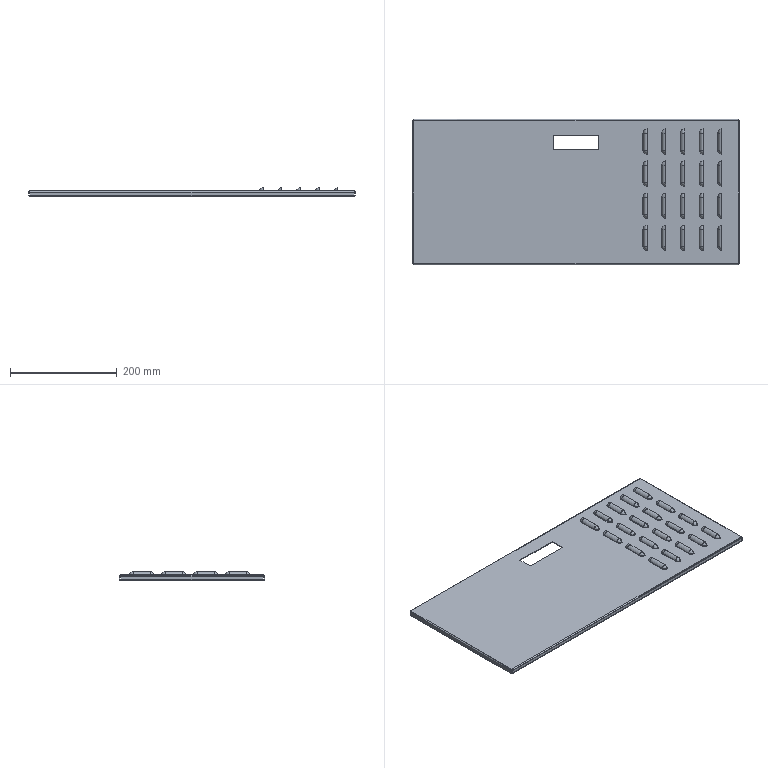Part | SolidWorks | features EdgeFlange 2, Cut 1, FlatPattern 1, FormToolInstance 1, LPattern 1, SMBaseFlange 1, SheetMetal 1 | 1 solid | 354 faces | box 610.973 x 271.523 x 15.997 mm | volume 290304 mm3 | cylinder 96 | plane 82 | torus 80 | sphere 80 | spline 16 | commonest cylinder face diameters 1 x20 4 x20 12 x20 15 x20 1.473 x8 4.473 x8